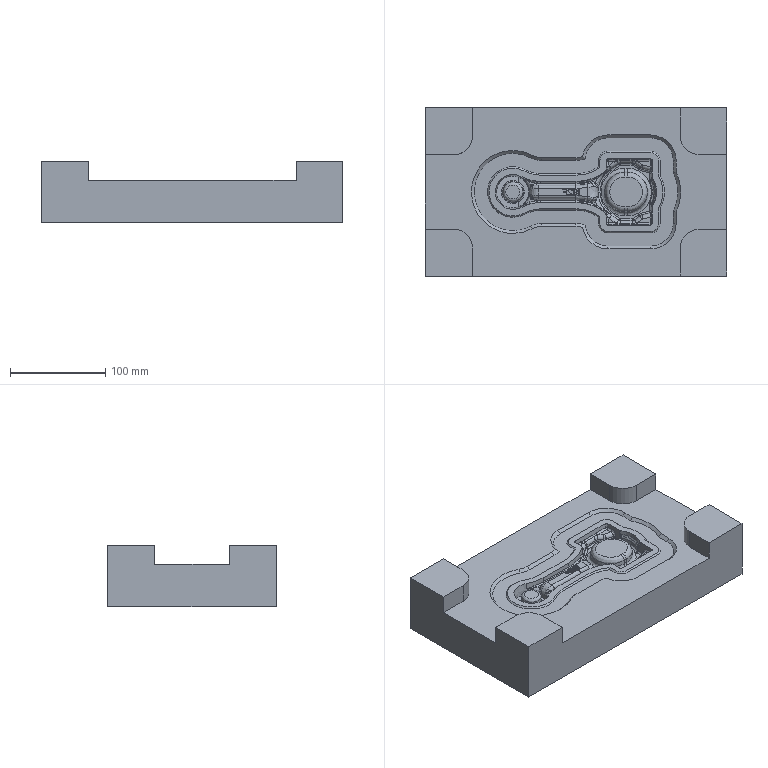NC program | NX | posted with a generic post | part box 317 x 177 x 65 mm
Lines 3445 to 4333 of 8842:
(CAVITY_MILL_COPY , TOOL : D12)
N6888 M6
N6890 G54
N6892 G17 G0 G90 X56.854 Y-0.717 S3000 M3
N6894 G43 Z10. H0
N6896 Z-19.8
N6898 G94 G3 X48.387 Y-3.113 Z-20.298 R-4.8 F2500.
N6900 G2 X50.906 Y-6.443 R53.174
N6902 G1 X53.992
N6904 G2 X56.323 Y0. R53.183
N6906 X53.991 Y6.443 R53.153
N6908 G1 X50.889
N6910 G2 X45.613 Y0.01 R53.277
N6912 X48.386 Y-3.113 R53.174
N6914 G1 X42.355 Y-8.059
N6916 G2 X46.623 Y-14.243 R45.374
N6918 G1 X60.23
N6920 G2 X63.991 Y-1.973 R45.383
N6922 G3 X63.996 Y1.962 R4.609
N6924 G2 X60.229 Y14.243 R45.353
N6926 G1 X46.607
N6928 G2 X33.762 Y0.006 R45.477
N6930 X42.355 Y-8.059 R45.374
N6932 G1 X36.324 Y-13.005
N6934 G2 X41.812 Y-22.043 R37.574
N6936 G1 X67.482
N6938 Y-21.162
N6940 G2 X71.048 Y-5.295 R37.583
N6942 G3 X71.054 Y5.283 R12.409
N6944 G2 X67.481 Y21.164 R37.553
N6946 G1 Y22.043
N6948 X41.801
N6950 G2 X17.527 Y0.676 R37.677
N6952 X14.947 Y-0.003 R64.013
N6954 G1 X8.985 Y-0.674
N6956 G3 X0.008 Y-0.014 R61.627
N6958 G1 X-35.639
N6960 X-35.667
N6962 X-36.637 Y-0.019
N6964 G3 X-44.679 Y-0.645 R57.686
N6966 X-44.678 Y0.645 R6.
N6968 X-36.557 Y0.016 R57.722
N6970 G1 X0.017 Y0.014
N6972 G3 X8.986 Y0.675 R62.213
N6974 X8.985 Y-0.674 R6.
N6976 G1 X14.947 Y-0.003
N6978 G2 X18.459 Y-0.962 R63.427
N6980 X36.324 Y-13.005 R37.574
N6982 G1 X30.293 Y-17.952
N6984 G2 X36.213 Y-29.843 R29.774
N6986 G1 X75.281
N6988 X75.282 Y-21.175
N6990 G2 X78.108 Y-8.612 R29.783
N6992 G3 X78.112 Y8.604 R20.209
N6994 G2 X75.281 Y21.179 R29.753
N6996 G1 X75.275 Y29.843
N6998 X36.209
N7000 G2 X15.385 Y8.176 R29.877
N7002 X0.017 Y6.014 R56.213
N7004 G1 X-36.556 Y6.016
N7006 G2 X-59.827 Y11.74 R51.722
N7008 G1 X-65.863 Y0.001
N7010 G2 X-66.319 Y0.238 R64.922
N7012 G3 X-66.319 Y-0.236 R-0.257
N7014 G2 X-65.863 Y0.001 R64.886
N7016 G1 X-63.394 Y4.803
N7018 G2 X-63.882 Y5.057 R59.522
N7020 G3 X-63.882 Y-5.055 R-5.657
N7022 G2 X-50.644 Y0. R59.486
N7024 X-63.394 Y4.803 R59.522
N7026 G1 X-59.827 Y11.74
N7028 G2 X-60.301 Y11.987 R51.722
N7030 G3 X-60.301 Y-11.985 R-13.457
N7032 G2 X-36.609 Y-6.019 R51.686
N7034 G1 X-35.639 Y-6.014
N7036 X0.006
N7038 G2 X16.161 Y-8.416 R55.627
N7040 X30.293 Y-17.952 R29.774
N7042 G1 X24.262 Y-22.898
N7044 G2 X29.02 Y-33.696 R21.974
N7046 G3 X33.759 Y-37.643 R4.684
N7048 G1 X78.24
N7050 G3 X83.075 Y-33.111 R4.677
N7052 G1 X83.081 Y-32.426
N7054 X83.082 Y-21.191
N7056 G2 X85.167 Y-11.931 R21.983
N7058 G3 X85.17 Y11.924 R28.009
N7060 G2 X83.081 Y21.195 R21.953
N7062 G1 X83.073 Y33.136
N7064 G3 X78.239 Y37.643 R4.677
N7066 G1 X33.759
N7068 G3 X29.015 Y33.651 R4.684
N7070 G2 X13.242 Y15.676 R22.077
N7072 X0.012 Y13.814 R48.413
N7074 G1 X-36.525 Y13.816
N7076 G2 X-56.701 Y18.907 R43.922
N7078 G3 X-56.701 Y-18.905 R-21.257
N7080 G2 X-36.559 Y-13.819 R43.886
N7082 G1 X-35.621 Y-13.814
N7084 X0.004
N7086 G2 X13.86 Y-15.869 R47.827
N7088 X24.262 Y-22.898 R21.974
N7090 G1 X18.231 Y-27.844
N7092 G2 X21.305 Y-34.846 R14.174
N7094 G3 X33.81 Y-45.443 R12.484
N7096 G1 X78.167
N7098 G3 X90.874 Y-33.249 R12.477
N7100 G1 X90.881 Y-32.464
N7102 X90.882 Y-21.209
N7104 G2 X92.226 Y-15.249 R14.183
N7106 G3 X92.227 Y15.245 R35.809
N7108 G2 X90.881 Y21.213 R14.153
N7110 G1 X90.873 Y33.246
N7112 G3 X78.167 Y45.443 R12.477
N7114 G1 X33.81
N7116 G3 X21.3 Y34.8 R12.484
N7118 G2 X11.1 Y23.176 R14.277
N7120 X0.006 Y21.614 R40.613
N7122 G1 X-36.491 Y21.616
N7124 G2 X-53.091 Y25.821 R36.122
N7126 G3 X-53.091 Y-25.819 R-29.057
N7128 G2 X-36.506 Y-21.619 R36.086
N7130 G1 X-35.602 Y-21.614
N7132 X0.002
N7134 G2 X11.555 Y-23.321 R40.027
N7136 X18.231 Y-27.844 R14.174
N7138 G1 X12.2 Y-32.791
N7140 G2 X13.586 Y-35.969 R6.374
N7142 G3 X33.848 Y-53.243 R20.284
N7144 G1 X78.112
N7146 G3 X98.673 Y-33.369 R20.277
N7148 G1 X98.681 Y-32.502
N7150 X98.682 Y-21.235
N7152 G2 X99.286 Y-18.566 R6.383
N7154 G3 X99.285 Y18.566 R43.609
N7156 G2 X98.681 Y21.235 R6.353
N7158 G1 Y32.502
N7160 X98.672 Y33.369
N7162 G3 X78.112 Y53.243 R20.277
N7164 G1 X33.848
N7166 G3 X13.585 Y35.95 R20.284
N7168 G2 X8.957 Y30.676 R6.477
N7170 X0. Y29.414 R32.813
N7172 G1 X-36.452 Y29.416
N7174 G2 X-49.471 Y32.73 R28.322
N7176 G3 X-49.471 Y-32.728 R-36.857
N7178 G2 X-36.452 Y-29.418 R28.286
N7180 G1 X-35.584 Y-29.414
N7182 X0.
N7184 G2 X9.234 Y-30.768 R32.227
N7186 X12.2 Y-32.791 R6.374
N7188 G1 X16.839 Y-28.986
N7190 Z-20.098
N7192 G0 Z10.
N7194 X57.197 Y-0.589
N7196 Z-20.098
N7198 G3 X48.724 Y-2.966 Z-20.596 R-4.8
N7200 G2 X51.128 Y-6.146 R53.161
N7202 G1 X53.761
N7204 G2 X55.995 Y0. R53.188
N7206 X53.76 Y6.145 R53.144
N7208 G1 X51.087
N7210 G2 X46.089 Y0.025 R53.374
N7212 X48.724 Y-2.966 R53.161
N7214 G1 X42.683 Y-7.899
N7216 G2 X46.852 Y-13.946 R45.361
N7218 G1 X59.968
N7220 G2 X63.719 Y-1.851 R45.388
N7222 G3 X63.724 Y1.841 R4.311
N7224 G2 X59.967 Y13.945 R45.344
N7226 G1 X46.818
N7228 G2 X34.334 Y0.018 R45.574
N7230 X42.683 Y-7.899 R45.361
N7232 G1 X36.641 Y-12.832
N7234 G2 X42.05 Y-21.745 R37.561
N7236 G1 X67.183 Y-21.746
N7238 Y-21.269
N7240 G2 X70.771 Y-5.183 R37.588
N7242 G3 X70.777 Y5.171 R12.111
N7244 G2 X67.183 Y21.283 R37.544
N7246 G1 Y21.745
N7248 X42.027
N7250 G2 X18.012 Y0.513 R37.774
N7252 X16.16 Y-0.001 R64.016
N7254 G1 X8.817 Y0.
N7256 X16.16 Y-0.001
N7258 G2 X18.971 Y-0.807 R63.835
N7260 X36.641 Y-12.832 R37.561
N7262 G1 X30.599 Y-17.766
N7264 G2 X36.462 Y-29.545 R29.761
N7266 G1 X74.983 Y-29.546
N7268 Y-21.262
N7270 G2 X77.825 Y-8.513 R29.788
N7272 G3 X77.83 Y8.502 R19.911
N7274 G2 X74.983 Y21.274 R29.744
N7276 G1 Y29.545
N7278 X36.457
N7280 G2 X15.813 Y7.996 R29.974
N7282 X0.011 Y5.716 R56.216
N7284 G1 X-36.553 Y5.718
N7286 G2 X-49.781 Y7.528 R51.983
N7288 G1 X-51.822 Y0.
N7290 G2 X-63.942 Y4.754 R59.783
N7292 G3 X-63.94 Y-4.752 R-5.359
N7294 G2 X-51.822 Y0. R59.8
N7296 G1 X-44.58 Y-0.001
N7298 X-51.822 Y0.
N7300 X-49.781 Y7.528
N7302 G2 X-60.328 Y11.666 R51.983
N7304 G3 X-60.326 Y-11.664 R-13.159
N7306 G2 X-36.612 Y-5.721 R52.
N7308 G1 X-35.639 Y-5.716
N7310 X0.009
N7312 G2 X16.623 Y-8.245 R56.035
N7314 X30.599 Y-17.766 R29.761
N7316 G1 X24.557 Y-22.699
N7318 G2 X29.293 Y-33.527 R21.961
N7320 G3 X31.812 Y-36.943 R4.463
N7322 X33.61 Y-37.345 R4.222
N7324 G1 X78.315 Y-37.346
N7326 G3 X82.776 Y-33.103 R4.381
N7328 G1 X82.783 Y-32.42
N7330 Y-21.255
N7332 G2 X84.879 Y-11.841 R21.988
N7334 G3 X84.884 Y11.832 R27.711
N7336 G2 X82.783 Y21.263 R21.944
N7338 G1 Y32.404
N7340 X82.774 Y33.096
N7342 G3 X78.243 Y37.345 R4.375
N7344 G1 X33.755
N7346 G3 X29.31 Y33.593 R4.377
N7348 G2 X13.614 Y15.48 R22.174
N7350 X0.008 Y13.516 R48.416
N7352 G1 X-36.523 Y13.518
N7354 G2 X-56.711 Y18.577 R44.183
N7356 G3 X-56.709 Y-18.574 R-20.959
N7358 G2 X-36.56 Y-13.52 R44.2
N7360 G1 X-35.621 Y-13.516
N7362 X0.005
N7364 G2 X14.273 Y-15.683 R48.235
N7366 X24.557 Y-22.699 R21.961
N7368 G1 X18.515 Y-27.632
N7370 G2 X21.569 Y-34.615 R14.161
N7372 G3 X28.491 Y-44.001 R12.263
N7374 X33.61 Y-45.145 R12.022
N7376 G1 X78.168
N7378 G3 X90.575 Y-33.245 R12.181
N7380 G1 X90.583 Y-32.461
N7382 Y-21.246
N7384 G2 X91.934 Y-15.168 R14.188
N7386 G3 X91.937 Y15.162 R35.511
N7388 G2 X90.583 Y21.251 R14.144
N7390 G1 Y32.453
N7392 X90.573 Y33.239
N7394 G3 X78.168 Y45.145 R12.175
N7396 G1 X33.808
N7398 G3 X21.59 Y34.705 R12.177
N7400 G2 X11.415 Y22.964 R14.374
N7402 X0.004 Y21.316 R40.616
N7404 G1 X-36.49 Y21.318
N7406 G2 X-53.091 Y25.486 R36.383
N7408 G3 X-53.09 Y-25.484 R-28.759
N7410 G2 X-36.507 Y-21.32 R36.4
N7412 G1 X-35.602 Y-21.316
N7414 X0.003
N7416 G2 X11.917 Y-23.119 R40.435
N7418 X18.515 Y-27.632 R14.161
N7420 G1 X12.473 Y-32.566
N7422 G2 X13.845 Y-35.702 R6.361
N7424 G3 X25.169 Y-51.058 R20.063
N7426 X33.61 Y-52.945 R19.822
N7428 G1 X78.112
N7430 G3 X98.374 Y-33.369 R19.981
N7432 G1 X98.383 Y-32.502
N7434 Y-21.235
N7436 G2 X98.99 Y-18.493 R6.388
N7438 G3 X98.99 Y18.493 R43.311
N7440 G2 X98.383 Y21.235 R6.344
N7442 G1 Y32.502
N7444 X98.372 Y33.369
N7446 G3 X78.112 Y52.945 R19.975
N7448 G1 X33.848
N7450 G3 X13.869 Y35.817 R19.977
N7452 G2 X9.216 Y30.447 R6.574
N7454 X0. Y29.116 R32.816
N7456 G1 X-36.452 Y29.118
N7458 G2 X-49.471 Y32.395 R28.583
N7460 G3 X-49.471 Y-32.394 R-36.559
N7462 G2 X-36.452 Y-29.12 R28.6
N7464 G1 X-35.584 Y-29.116
N7466 X0.
N7468 G2 X9.547 Y-30.551 R32.635
N7470 X12.473 Y-32.566 R6.361
N7472 G1 X17.121 Y-28.771
N7474 Z-20.396
N7476 G0 Z-19.998
N7478 X53.117 Y-4.976
N7480 Z-20.396
N7482 G3 X49.073 Y2.839 Z-20.895 R-4.8
N7484 G2 X46.594 Y0. R53.195
N7486 X51.344 Y-5.847 R53.175
N7488 G1 X53.532
N7490 G2 X55.668 Y-0.001 R53.202
N7492 X53.53 Y5.847 R53.144
N7494 G1 X51.343
N7496 G2 X49.073 Y2.839 R53.195
N7498 G1 X43.018 Y7.757
N7500 G2 X34.937 Y-0.001 R45.395
N7502 X47.076 Y-13.647 R45.375
N7504 G1 X59.708
N7506 G2 X63.453 Y-1.717 R45.402
N7508 G3 X63.452 Y1.718 R4.013
N7510 G2 X59.706 Y13.647 R45.344
N7512 G1 X47.076
N7514 G2 X43.018 Y7.757 R45.395
N7516 G1 X36.963 Y12.674
N7518 G2 X18.649 Y0.385 R37.595
N7520 X17.313 Y-0.002 R64.817
N7522 G1 X10.39 Y0.
N7524 X17.313 Y-0.002
N7526 G2 X18.767 Y-0.428 R64.512
N7528 X42.285 Y-21.447 R37.575
N7530 G1 X66.885
N7532 G2 X70.502 Y-5.055 R37.602
N7534 G3 X70.501 Y5.058 R11.813
N7536 G2 X66.884 Y21.447 R37.544
N7538 G1 X42.285
N7540 G2 X36.963 Y12.674 R37.595
N7542 G1 X30.909 Y17.591
N7544 G2 X16.394 Y7.852 R29.795
N7546 X0.027 Y5.418 R57.018
N7548 G1 X-36.555 Y5.421
N7550 G2 X-50.748 Y7.491 R52.298
N7552 G1 X-52.921 Y0.
N7554 G2 X-63.986 Y4.442 R60.098
N7556 G3 X-71.477 Y0. R5.062
N7558 X-63.986 Y-4.442 R5.062
N7560 G2 X-52.921 Y0. R60.087
N7562 G1 X-46.098
N7564 X-52.921
N7566 X-50.748 Y7.491
N7568 G2 X-60.343 Y11.339 R52.298
N7570 G3 X-79.277 Y0. R12.862
N7572 X-60.343 Y-11.339 R12.862
N7574 G2 X-36.612 Y-5.422 R52.287
N7576 G1 X-35.64 Y-5.418
N7578 X0.021
N7580 G2 X16.49 Y-7.888 R56.712
N7582 X36.71 Y-29.247 R29.775
N7584 G1 X74.685
N7586 Y-21.147
N7588 G2 X77.552 Y-8.393 R29.802
N7590 G3 X77.549 Y8.398 R19.613
N7592 G2 X74.685 Y21.13 R29.744
N7594 G1 X74.678 Y29.247
N7596 X36.71
N7598 G2 X30.909 Y17.591 R29.795
N7600 G1 X24.854 Y22.509
N7602 G2 X14.139 Y15.319 R21.995
N7604 X0.019 Y13.218 R49.218
N7606 G1 X-36.524 Y13.221
N7608 G2 X-56.711 Y18.242 R44.498
N7610 G3 X-87.077 Y0. R20.662
N7612 X-56.711 Y-18.242 R20.662
N7614 G2 X-36.561 Y-13.222 R44.487
N7616 G1 X-35.621 Y-13.218
N7618 X0.014
N7620 G2 X14.214 Y-15.348 R48.912
N7622 X29.491 Y-32.855 R21.975
N7624 G1 X29.602 Y-33.537
N7626 G3 X33.759 Y-37.047 R4.094
N7628 G1 X78.238
N7630 G3 X82.477 Y-33.089 R4.093
N7632 G1 X82.485 Y-32.414
N7634 Y-21.147
N7636 G2 X84.601 Y-11.731 R22.002
N7638 G3 X84.598 Y11.738 R27.413
N7640 G2 X82.485 Y21.134 R21.944
N7642 G1 X82.475 Y33.078
N7644 G3 X78.241 Y37.047 R4.085
N7646 G1 X33.755
N7648 G3 X29.601 Y33.497 R4.078
N7650 G1 X29.468 Y32.707
N7652 G2 X24.854 Y22.509 R21.995
N7654 G1 X18.799 Y27.426
N7656 G2 X11.884 Y22.786 R14.195
N7658 X0.01 Y21.018 R41.418
N7660 G1 X-36.49 Y21.021
N7662 G2 X-53.088 Y25.15 R36.698
N7664 G3 X-94.877 Y0. R28.462
N7666 X-53.088 Y-25.149 R28.462
N7668 G2 X-36.507 Y-21.022 R36.687
N7670 G1 X-35.603 Y-21.018
N7672 X0.008
N7674 G2 X11.937 Y-22.809 R41.112
N7676 X21.792 Y-34.101 R14.175
N7678 G1 X21.896 Y-34.748
N7680 G3 X33.81 Y-44.847 R11.894
N7682 G1 X78.166
N7684 G3 X90.276 Y-33.238 R11.893
N7686 G1 X90.285 Y-32.458
N7688 Y-21.147
N7690 G2 X91.651 Y-15.069 R14.202
N7692 G3 X91.647 Y15.078 R35.213
N7694 G2 X90.285 Y21.134 R14.144
N7696 G1 Y32.446
N7698 X90.273 Y33.229
N7700 G3 X78.167 Y44.847 R11.885
N7702 G1 X33.808
N7704 G3 X21.898 Y34.724 R11.878
N7706 G1 X21.777 Y34.008
N7708 G2 X18.799 Y27.426 R14.195
N7710 G1 X12.745 Y32.344
N7712 G2 X9.629 Y30.253 R6.395
N7714 X0. Y28.818 R33.618
N7716 G1 X-36.452 Y28.821
N7718 G2 X-49.471 Y32.06 R28.898
N7720 G3 X-49.471 Y-32.06 R-36.262
N7722 G2 X-36.452 Y-28.822 R28.887
N7724 G1 X-35.584 Y-28.818
N7726 X0.
N7728 G2 X9.66 Y-30.269 R33.312
N7730 X14.092 Y-35.348 R6.375
N7732 G1 X14.192 Y-35.969
N7734 G3 X33.848 Y-52.647 R19.694
N7736 G1 X78.112
N7738 G3 X98.075 Y-33.369 R19.693
N7740 G1 X98.085 Y-32.502
N7742 Y-21.147
N7744 G2 X98.701 Y-18.407 R6.402
N7746 G3 X98.696 Y18.418 R43.013
N7748 G2 X98.085 Y21.134 R6.344
N7750 G1 Y32.502
N7752 X98.072 Y33.369
N7754 G3 X78.112 Y52.647 R19.685
N7756 G1 X33.848
N7758 G3 X14.198 Y35.969 R19.678
N7760 G1 X14.086 Y35.309
N7762 G2 X12.745 Y32.344 R6.395
N7764 G1 X17.402 Y28.561
N7766 Z-20.695
N7768 G0 Z-20.296
N7770 X53.482 Y-5.109
N7772 Z-20.695
N7774 G3 X49.422 Y2.698 Z-21.193 R-4.8
N7776 G2 X47.085 Y-0.001 R53.134
N7778 X51.573 Y-5.549 R53.136
N7780 G1 X53.308
N7782 G2 X55.342 Y-0.001 R53.366
N7784 X53.306 Y5.549 R53.306
N7786 G1 X51.573
N7788 G2 X49.422 Y2.699 R53.134
N7790 G1 X43.358 Y7.604
N7792 G2 X35.514 Y0. R45.334
N7794 X47.314 Y-13.349 R45.336
N7796 G1 X59.453 Y-13.35
N7798 G2 X63.182 Y-1.592 R45.566
N7800 G3 X63.181 Y1.592 R3.714
N7802 G2 X59.452 Y13.349 R45.506
N7804 G1 X47.315
N7806 G2 X43.358 Y7.604 R45.334
N7808 G1 X37.293 Y12.509
N7810 G2 X21.045 Y0.879 R37.534
N7812 X18.378 Y0.006 R62.632
N7814 G1 X11.759 Y-0.009
N7816 X18.378 Y0.006
N7818 G2 X18.994 Y-0.179 R65.178
N7820 G1 X19.117 Y-0.217
N7822 X20.977 Y-0.855
N7824 G2 X42.532 Y-21.149 R37.536
N7826 G1 X66.587 Y-21.15
N7828 G2 X70.229 Y-4.934 R37.766
N7830 G3 X70.228 Y4.937 R11.514
N7832 G2 X66.586 Y21.149 R37.706
N7834 G1 X42.533
N7836 G2 X37.293 Y12.509 R37.534
N7838 G1 X31.229 Y17.415
N7840 G2 X18.403 Y8.218 R29.734
N7842 X0.229 Y5.12 R54.832
N7844 G1 X-36.153
N7846 G2 X-51.658 Y7.454 R52.648
N7848 G1 X-53.955 Y0.
N7850 G2 X-63.075 Y3.646 R60.448
N7852 G1 X-64.273 Y4.242
N7854 G3 X-71.177 Y-0.002 R4.756
N7856 X-64.301 Y-4.26 R4.756
N7858 G1 X-63.242 Y-3.729
N7860 G2 X-53.955 Y0. R60.434
N7862 G1 X-47.405
N7864 X-53.955
N7866 X-51.658 Y7.454
N7868 G2 X-59.601 Y10.629 R52.648
N7870 G1 X-60.786 Y11.219
N7872 G3 X-60.813 Y-11.236 R-12.556
N7874 G1 X-59.746 Y-10.702
N7876 G2 X-36.157 Y-5.12 R52.634
N7878 G1 X0.042
N7880 G2 X16.709 Y-7.637 R57.378
N7882 G1 X18.366 Y-8.205
N7884 G2 X36.968 Y-28.949 R29.736
N7886 G1 X74.387 Y-28.95
N7888 Y-21.117
N7890 G2 X77.277 Y-8.276 R29.966
N7892 G3 X77.275 Y8.281 R19.314
N7894 G2 X74.387 Y21.094 R29.906
N7896 G1 X74.379 Y28.949
N7898 X36.969
N7900 G2 X31.229 Y17.415 R29.734
N7902 G1 X25.165 Y22.32
N7904 G2 X15.756 Y15.556 R21.934
N7906 X0.229 Y12.92 R47.032
N7908 G1 X-36.153
N7910 G2 X-56.127 Y17.613 R44.848
N7912 G1 X-57.302 Y18.198
N7914 G3 X-57.322 Y-18.212 R-20.356
N7916 G1 X-56.25 Y-17.674
N7918 G2 X-36.157 Y-12.92 R44.834
N7920 G1 X0.022
N7922 G2 X14.309 Y-15.06 R49.578
N7924 G1 X15.743 Y-15.552
N7926 G2 X29.875 Y-33.387 R21.936
N7928 G3 X33.684 Y-36.749 R3.84
N7930 G1 X78.333 Y-36.75
N7932 G3 X82.179 Y-33.082 R3.794
N7934 G1 X82.187 Y-32.409
N7936 Y-21.117
N7938 G2 X84.325 Y-11.619 R22.166
N7940 G3 X84.321 Y11.625 R27.114
N7942 G2 X82.187 Y21.099 R22.106
N7944 G1 X82.175 Y33.11
N7946 G3 X78.242 Y36.749 R3.788
N7948 G1 X33.769
N7950 G3 X29.835 Y33.084 R3.843
N7952 G2 X25.165 Y22.32 R21.934
N7954 G1 X19.1 Y27.226
N7956 G2 X13.099 Y22.89 R14.134
N7958 X0.229 Y20.72 R39.232
N7960 G1 X-36.153
N7962 G2 X-52.653 Y24.597 R37.048
N7964 G1 X-53.82 Y25.177
N7966 G3 X-53.831 Y-25.187 R-28.156
N7968 G1 X-52.755 Y-24.647
N7970 G2 X-36.157 Y-20.72 R37.034
N7972 G1 X0.012
N7974 G2 X11.921 Y-22.487 R41.778
N7976 G1 X13.101 Y-22.891
N7978 G2 X22.135 Y-34.358 R14.136
N7980 G3 X33.684 Y-44.549 R11.64
N7982 G1 X78.223
N7984 G3 X89.977 Y-33.235 R11.594
N7986 G1 X89.987 Y-32.456
N7988 Y-21.117
N7990 G2 X91.372 Y-14.961 R14.366
N7992 G3 X91.368 Y14.97 R34.914
N7994 G2 X89.987 Y21.103 R14.306
N7996 G1 X89.975 Y33.224
N7998 G3 X78.168 Y44.549 R11.588
N8000 G1 X33.815
N8002 G3 X22.091 Y34.037 R11.643
N8004 G2 X19.1 Y27.226 R14.134
N8006 G1 X13.034 Y32.132
N8008 G2 X10.415 Y30.216 R6.334
N8010 X0.229 Y28.52 R31.432
N8012 G1 X-36.153
N8014 G2 X-49.179 Y31.58 R29.248
N8016 G1 X-50.339 Y32.157
N8018 G3 X-50.339 Y-32.161 R-35.956
N8020 G1 X-49.259 Y-31.62
N8022 G2 X-36.157 Y-28.52 R29.234
N8024 G1 X0.
N8026 G2 X9.547 Y-29.919 R33.978
N8028 G1 X10.415 Y-30.216
N8030 G2 X14.396 Y-35.329 R6.336
N8032 G3 X33.684 Y-52.349 R19.44
N8034 G1 X78.112
N8036 G3 X97.776 Y-33.369 R19.394
N8038 G1 X97.787 Y-32.502
N8040 Y-21.117
N8042 G2 X98.42 Y-18.303 R6.566
N8044 G3 X98.415 Y18.314 R42.714
N8046 G2 X97.787 Y21.103 R6.506
N8048 G1 Y32.502
N8050 X97.773 Y33.369
N8052 G3 X78.112 Y52.349 R19.388
N8054 G1 X33.848
N8056 G3 X14.362 Y35.102 R19.443
N8058 G2 X13.034 Y32.132 R6.334
N8060 G1 X17.699 Y28.359
N8062 Z-20.993
N8064 G0 Z-20.595
N8066 X60.593 Y1.642
N8068 Z-20.993
N8070 G3 X52.254 Y-1.168 Z-21.491 R-4.8
N8072 G2 X53.308 Y-2.385 R35.909
N8074 X54.48 Y-0.001 R32.921
N8076 X53.306 Y2.384 R32.888
N8078 X51.146 Y0. R35.913
N8080 X52.254 Y-1.168 R35.909
N8082 G1 X46.474 Y-6.406
N8084 G2 X50.837 Y-12.813 R28.109
N8086 G1 X58.458
N8088 G2 X62.506 Y-1.78 R25.121
N8090 G3 X62.503 Y1.785 R3.219
N8092 G2 X58.457 Y12.813 R25.088
N8094 G1 X50.836
N8096 G2 X41.799 Y2.277 R28.113
N8098 X38.349 Y0. R72.778
N8100 X41.805 Y-2.282 R72.778
N8102 X46.474 Y-6.406 R28.109
N8104 G1 X40.694 Y-11.643
N8106 G2 X45.41 Y-20.613 R20.309
N8108 G1 X66.09
N8110 Y-15.694
N8112 G2 X69. Y-6.102 R17.321
N8114 G3 X68.994 Y6.11 R11.019
N8116 G2 X66.09 Y15.697 R17.288
N8118 G1 Y20.613
N8120 X45.409
N8122 G2 X37.317 Y8.661 R20.313
N8124 X19.904 Y0. R64.978
N8126 G1 X13.561
N8128 X19.904
N8130 G2 X37.322 Y-8.665 R64.978
N8132 X40.694 Y-11.643 R20.309
N8134 G1 X34.914 Y-16.881
N8136 G2 X38.153 Y-25.293 R12.509
N8138 G1 Y-28.413
N8140 X73.89
N8142 Y-15.699
N8144 G2 X75.491 Y-10.426 R9.521
N8146 G3 X75.484 Y10.437 R18.819
N8148 G2 X73.89 Y15.699 R9.488
N8150 G1 Y28.413
N8152 X38.153
N8154 Y25.293
N8156 G2 X32.835 Y15.045 R12.513
N8158 X-0.002 Y4.676 R57.178
N8160 G1 X-36.393
N8162 G2 X-53.164 Y7.4 R53.252
N8164 G1 X-55.627 Y-0.001
N8166 G2 X-64.459 Y3.732 R61.052
N8168 G3 X-65.461 Y4.105 R4.215
N8170 X-64.458 Y-3.731 R-4.215
N8172 G2 X-55.627 Y-0.001 R61.143
N8174 G1 X-49.354
N8176 X-55.627
N8178 X-53.164 Y7.4
N8180 G2 X-60.86 Y10.651 R53.252
N8182 G3 X-60.86 Y-10.651 R-12.015
N8184 G2 X-36.393 Y-4.676 R53.343
N8186 G1 X-0.002
N8188 G2 X32.839 Y-15.048 R57.178
N8190 X34.914 Y-16.881 R12.509
N8192 G1 X39.36 Y-12.852
N8194 Z-21.291
N8196 G0 Z-20.893
N8198 X60.598 Y1.675
N8200 Z-21.291
N8202 G3 X52.262 Y-1.144 Z-21.789 R-4.8
N8204 G2 X53.297 Y-2.335 R35.876
N8206 X54.448 Y0. R32.832
N8208 X53.297 Y2.334 R32.828
N8210 X51.177 Y0. R35.877
N8212 X52.262 Y-1.144 R35.876
N8214 G1 X46.488 Y-6.388
N8216 G2 X50.851 Y-12.779 R28.076
N8218 G1 X58.432
N8220 G2 X62.479 Y-1.774 R25.032
N8222 G3 X62.479 Y1.774 R3.193
N8224 G2 X58.432 Y12.779 R25.028
N8226 G1 X50.851
N8228 G2 X41.837 Y2.285 R28.077
N8230 X38.378 Y0. R72.794
N8232 X41.836 Y-2.285 R72.794
N8234 X46.488 Y-6.388 R28.076
N8236 G1 X40.714 Y-11.631
N8238 G2 X45.431 Y-20.579 R20.276
N8240 G1 X66.064
N8242 Y-15.674
N8244 G2 X68.966 Y-6.106 R17.232
N8246 G3 X68.966 Y6.106 R10.993
N8248 G2 X66.064 Y15.675 R17.228
N8250 G1 Y20.579
N8252 X45.431
N8254 G2 X37.354 Y8.668 R20.277
N8256 X19.955 Y0. R64.994
N8258 G1 X13.621
N8260 X19.955
N8262 G2 X37.354 Y-8.668 R64.994
N8264 X40.714 Y-11.631 R20.276
N8266 G1 X34.939 Y-16.875
N8268 G2 X38.179 Y-25.259 R12.476
N8270 G1 Y-28.379
N8272 X73.864
N8274 Y-15.675
N8276 G2 X75.453 Y-10.437 R9.432
N8278 G3 X75.452 Y10.438 R18.793
N8280 G2 X73.864 Y15.675 R9.428
N8282 G1 Y28.379
N8284 X38.179
N8286 Y25.26
N8288 G2 X32.871 Y15.051 R12.477
N8290 X-0.002 Y4.66 R57.194
N8292 G1 X-36.474
N8294 G2 X-53.285 Y7.396 R52.81
N8296 G1 X-55.763 Y0.
N8298 G2 X-64.486 Y3.704 R60.61
N8300 G3 X-64.486 Y-3.704 R-4.178
N8302 G2 X-55.763 Y0. R60.61
N8304 G1 X-49.507
N8306 X-55.763
N8308 X-53.285 Y7.396
N8310 G2 X-60.883 Y10.622 R52.81
N8312 G3 X-60.883 Y-10.622 R-11.978
N8314 G2 X-36.474 Y-4.66 R52.81
N8316 G1 X-0.002
N8318 G2 X32.871 Y-15.051 R57.194
N8320 X34.939 Y-16.875 R12.476
N8322 G1 X39.381 Y-12.842
N8324 Z-21.589
N8326 G0 Z-21.191
N8328 X60.605 Y1.701
N8330 Z-21.589
N8332 G3 X52.271 Y-1.124 Z-22.088 R-4.8
N8334 G2 X53.289 Y-2.293 R35.876
N8336 X54.419 Y-0.002 R32.91
N8338 X53.287 Y2.29 R32.828
N8340 X51.204 Y0. R35.877
N8342 X52.271 Y-1.124 R35.876
N8344 G1 X46.5 Y-6.372
N8346 G2 X50.861 Y-12.745 R28.076
N8348 G1 X58.411
N8350 G2 X62.465 Y-1.748 R25.11
N8352 G3 X62.457 Y1.76 R3.167
N8354 G2 X58.409 Y12.745 R25.028
N8356 G1 X50.861
N8358 G2 X41.873 Y2.291 R28.077
N8360 X38.408 Y0. R72.81
N8362 X41.873 Y-2.291 R72.81
N8364 X46.5 Y-6.372 R28.076
N8366 G1 X40.73 Y-11.62
N8368 G2 X45.449 Y-20.545 R20.276
N8370 G1 X66.038
N8372 Y-15.657
N8374 G2 X68.957 Y-6.072 R17.31
N8376 G3 X68.942 Y6.094 R10.967
N8378 G2 X66.038 Y15.667 R17.228
N8380 G1 Y20.545
N8382 X45.449
N8384 G2 X37.388 Y8.673 R20.277
N8386 X20.006 Y0. R65.01
N8388 G1 X13.68
N8390 X20.006
N8392 G2 X37.388 Y-8.673 R65.01
N8394 X40.73 Y-11.62 R20.276
N8396 G1 X34.959 Y-16.868
N8398 G2 X38.206 Y-25.259 R12.476
N8400 G1 Y-28.345
N8402 X73.838
N8404 Y-15.667
N8406 G2 X75.446 Y-10.401 R9.51
N8408 G3 X75.427 Y10.428 R18.767
N8410 G2 X73.838 Y15.667 R9.428
N8412 G1 Y28.345
N8414 X38.206
N8416 Y25.259
N8418 G2 X32.902 Y15.054 R12.477
N8420 X-0.002 Y4.644 R57.21
N8422 G1 X-36.523
N8424 G2 X-53.372 Y7.396 R52.913
N8426 G1 X-55.855 Y0.001
N8428 G2 X-64.548 Y3.695 R60.713
N8430 G3 X-64.505 Y-3.673 R-4.141
N8432 G2 X-55.855 Y0.001 R60.613
N8434 G1 X-49.606
N8436 X-55.855
N8438 X-53.372 Y7.396
N8440 G2 X-60.975 Y10.629 R52.913
N8442 G3 X-60.906 Y-10.593 R-11.941
N8444 G2 X-36.523 Y-4.644 R52.813
N8446 G1 X-0.002
N8448 G2 X32.902 Y-15.054 R57.21
N8450 X34.959 Y-16.868 R12.476
N8452 G1 X39.398 Y-12.831
N8454 Z-21.888
N8456 G0 Z-21.489
N8458 X60.61 Y1.729
N8460 Z-21.888
N8462 G3 X52.278 Y-1.102 Z-22.386 R-4.8
N8464 G2 X53.278 Y-2.248 R35.877
N8466 X54.388 Y-0.001 R32.88
N8468 X53.277 Y2.246 R32.828
N8470 X51.23 Y0. R35.877
N8472 X52.278 Y-1.102 R35.877
N8474 G1 X46.512 Y-6.355
N8476 G2 X50.87 Y-12.711 R28.077
N8478 G1 X58.387
N8480 G2 X62.44 Y-1.739 R25.08
N8482 G3 X62.435 Y1.746 R3.141
N8484 G2 X58.386 Y12.711 R25.028
N8486 G1 X50.87
N8488 G2 X41.91 Y2.298 R28.077
N8490 X38.438 Y0. R72.825
N8492 X41.91 Y-2.298 R72.825
N8494 X46.512 Y-6.355 R28.077
N8496 G1 X40.745 Y-11.607
N8498 G2 X45.467 Y-20.511 R20.277
N8500 G1 X66.012
N8502 Y-15.653
N8504 G2 X68.928 Y-6.068 R17.28
N8506 G3 X68.919 Y6.082 R10.941
N8508 G2 X66.012 Y15.66 R17.228
N8510 G1 Y20.511
N8512 X45.467
N8514 G2 X37.422 Y8.677 R20.277
N8516 X20.057 Y0. R65.025
N8518 G1 X13.739
N8520 X20.057
N8522 G2 X37.421 Y-8.677 R65.025
N8524 X40.745 Y-11.607 R20.277
N8526 G1 X34.979 Y-16.86
N8528 G2 X38.232 Y-25.258 R12.477
N8530 G1 Y-28.311
N8532 X73.812
N8534 Y-15.659
N8536 G2 X75.414 Y-10.401 R9.48
N8538 G3 X75.403 Y10.418 R18.741
N8540 G2 X73.812 Y15.659 R9.428
N8542 G1 Y28.311
N8544 X38.232
N8546 Y25.258
N8548 G2 X32.933 Y15.056 R12.477
N8550 X-0.002 Y4.629 R57.225
N8552 G1 X-36.572
N8554 G2 X-53.462 Y7.394 R52.923
N8556 G1 X-55.95 Y0.001
N8558 G2 X-64.562 Y3.661 R60.723
N8560 G3 X-64.524 Y-3.641 R-4.105
N8562 G2 X-55.95 Y0.001 R60.617
N8564 G1 X-49.709 Y0.002
N8566 X-55.95 Y0.001
N8568 X-53.462 Y7.394
N8570 G2 X-60.991 Y10.596 R52.923
N8572 G3 X-60.929 Y-10.564 R-11.905
N8574 G2 X-36.572 Y-4.629 R52.817
N8576 G1 X-0.002
N8578 G2 X32.933 Y-15.056 R57.225
N8580 X34.979 Y-16.86 R12.477
N8582 G1 X39.414 Y-12.819
N8584 Z-22.186
N8586 G0 Z-20.893
N8588 X-60.28 Y7.155
N8590 Z-22.186
N8592 G3 X-60.364 Y-1.644 Z-22.684 R-4.8
N8594 G2 X-56.045 Y-0.001 R60.741
N8596 X-64.543 Y3.61 R60.541
N8598 G3 X-64.545 Y-3.611 R-4.068
N8600 G2 X-60.364 Y-1.644 R60.741
N8602 G1 X-57.314 Y-8.823
N8604 G2 X-47.555 Y-5.752 R52.941
N8606 X-47.706 Y0.433 R21.663
N8608 X-47.559 Y5.754 R14.36
N8610 X-60.953 Y10.534 R52.741
N8612 G3 X-60.953 Y-10.534 R-11.868
N8614 G2 X-57.314 Y-8.823 R52.941
N8616 G1 X-59.66 Y-3.301
N8618 Z-22.484
N8620 G0 Z-22.086
N8622 X-52.525 Y-6.993
N8624 Z-22.484
N8626 G1 X-50.373 Y-6.37 Z-22.543
N8628 X-48.603 Y-5.958 Z-22.59
N8630 X-48.809 Y-5.274 Z-22.609
N8632 X-48.966 Y-4.194 Z-22.638
N8634 X-48.983 Y-3.102 Z-22.666
N8636 X-48.752 Y-1.36 Z-22.712
N8638 X-48.753 Y1.373 Z-22.784
N8640 X-48.986 Y3.111 Z-22.83
N8642 X-48.969 Y4.199 Z-22.858
N8644 X-48.811 Y5.276 Z-22.887
N8646 X-48.605 Y5.955 Z-22.905
N8648 X-50.037 Y6.289 Z-22.944
N8650 X-51.449 Y6.7 Z-22.982
N8652 G2 X-54.249 Y7.598 R54.323
N8654 X-54.246 Y-7.593 R14.347
N8656 X-48.603 Y-5.958 R55.021
N8658 X-48.889 Y-2.394 R8.481